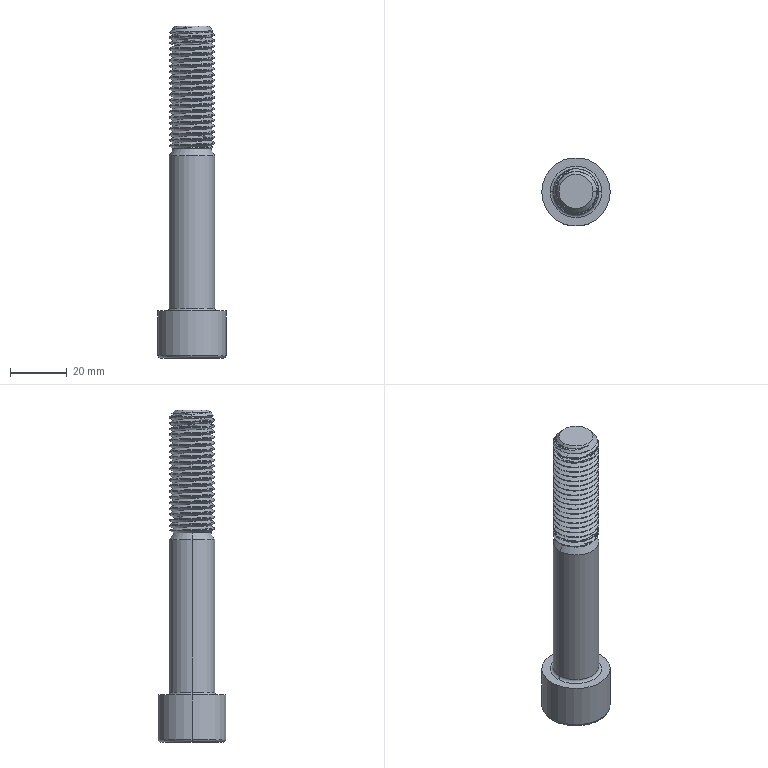Part | STEP file | Parafuso M16 - 100mm - DIN 912 (DIN EM ISO 4762) | 1 solid | 70 faces | box 24 x 24 x 116.5 mm | volume 24194 mm3 | cylinder 45 | plane 10 | cone 9 | torus 4 | spline 2 | commonest cylinder face diameters 16 x43 24 x2